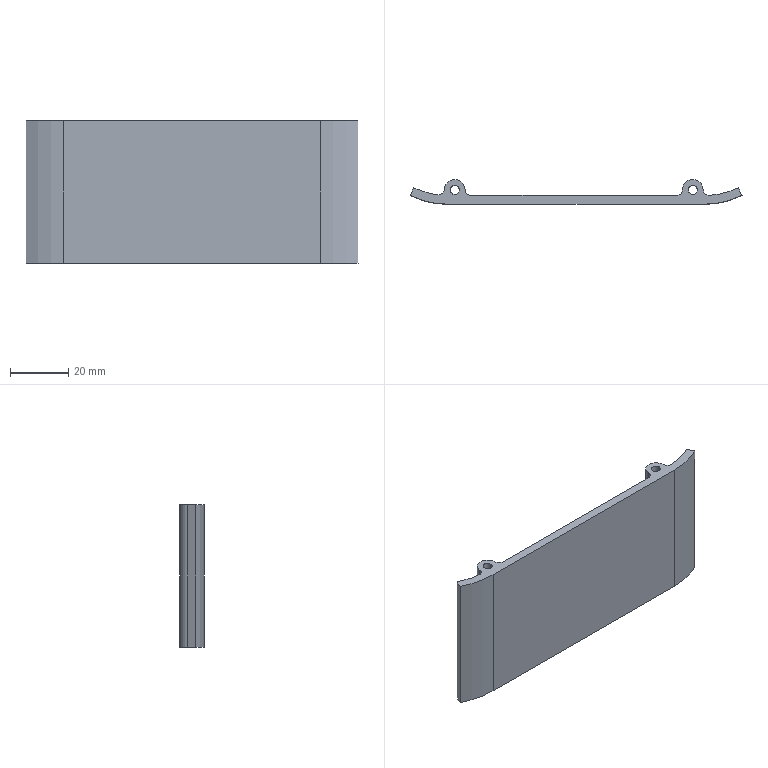Part | STEP file | Zaokr_glenie1_1 | 1 solid | 18 faces | box 114.379 x 8.512 x 49 mm | volume 19491 mm3 | cylinder 12 | plane 6 | commonest cylinder face diameters 4 x4 3.16 x2 7.16 x2 54 x2 60 x2